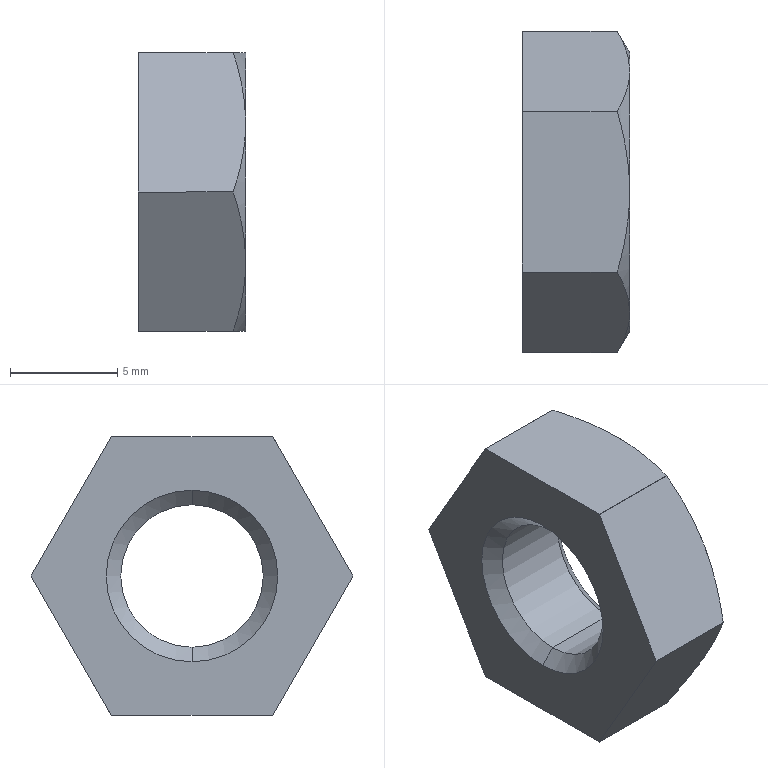Part | STEP file | 2_11 | 1 solid | 24 faces | box 5 x 15 x 13 mm | volume 545.323 mm3 | cone 10 | plane 8 | cylinder 6 | commonest cylinder face diameters 15 x4 6.647 x2